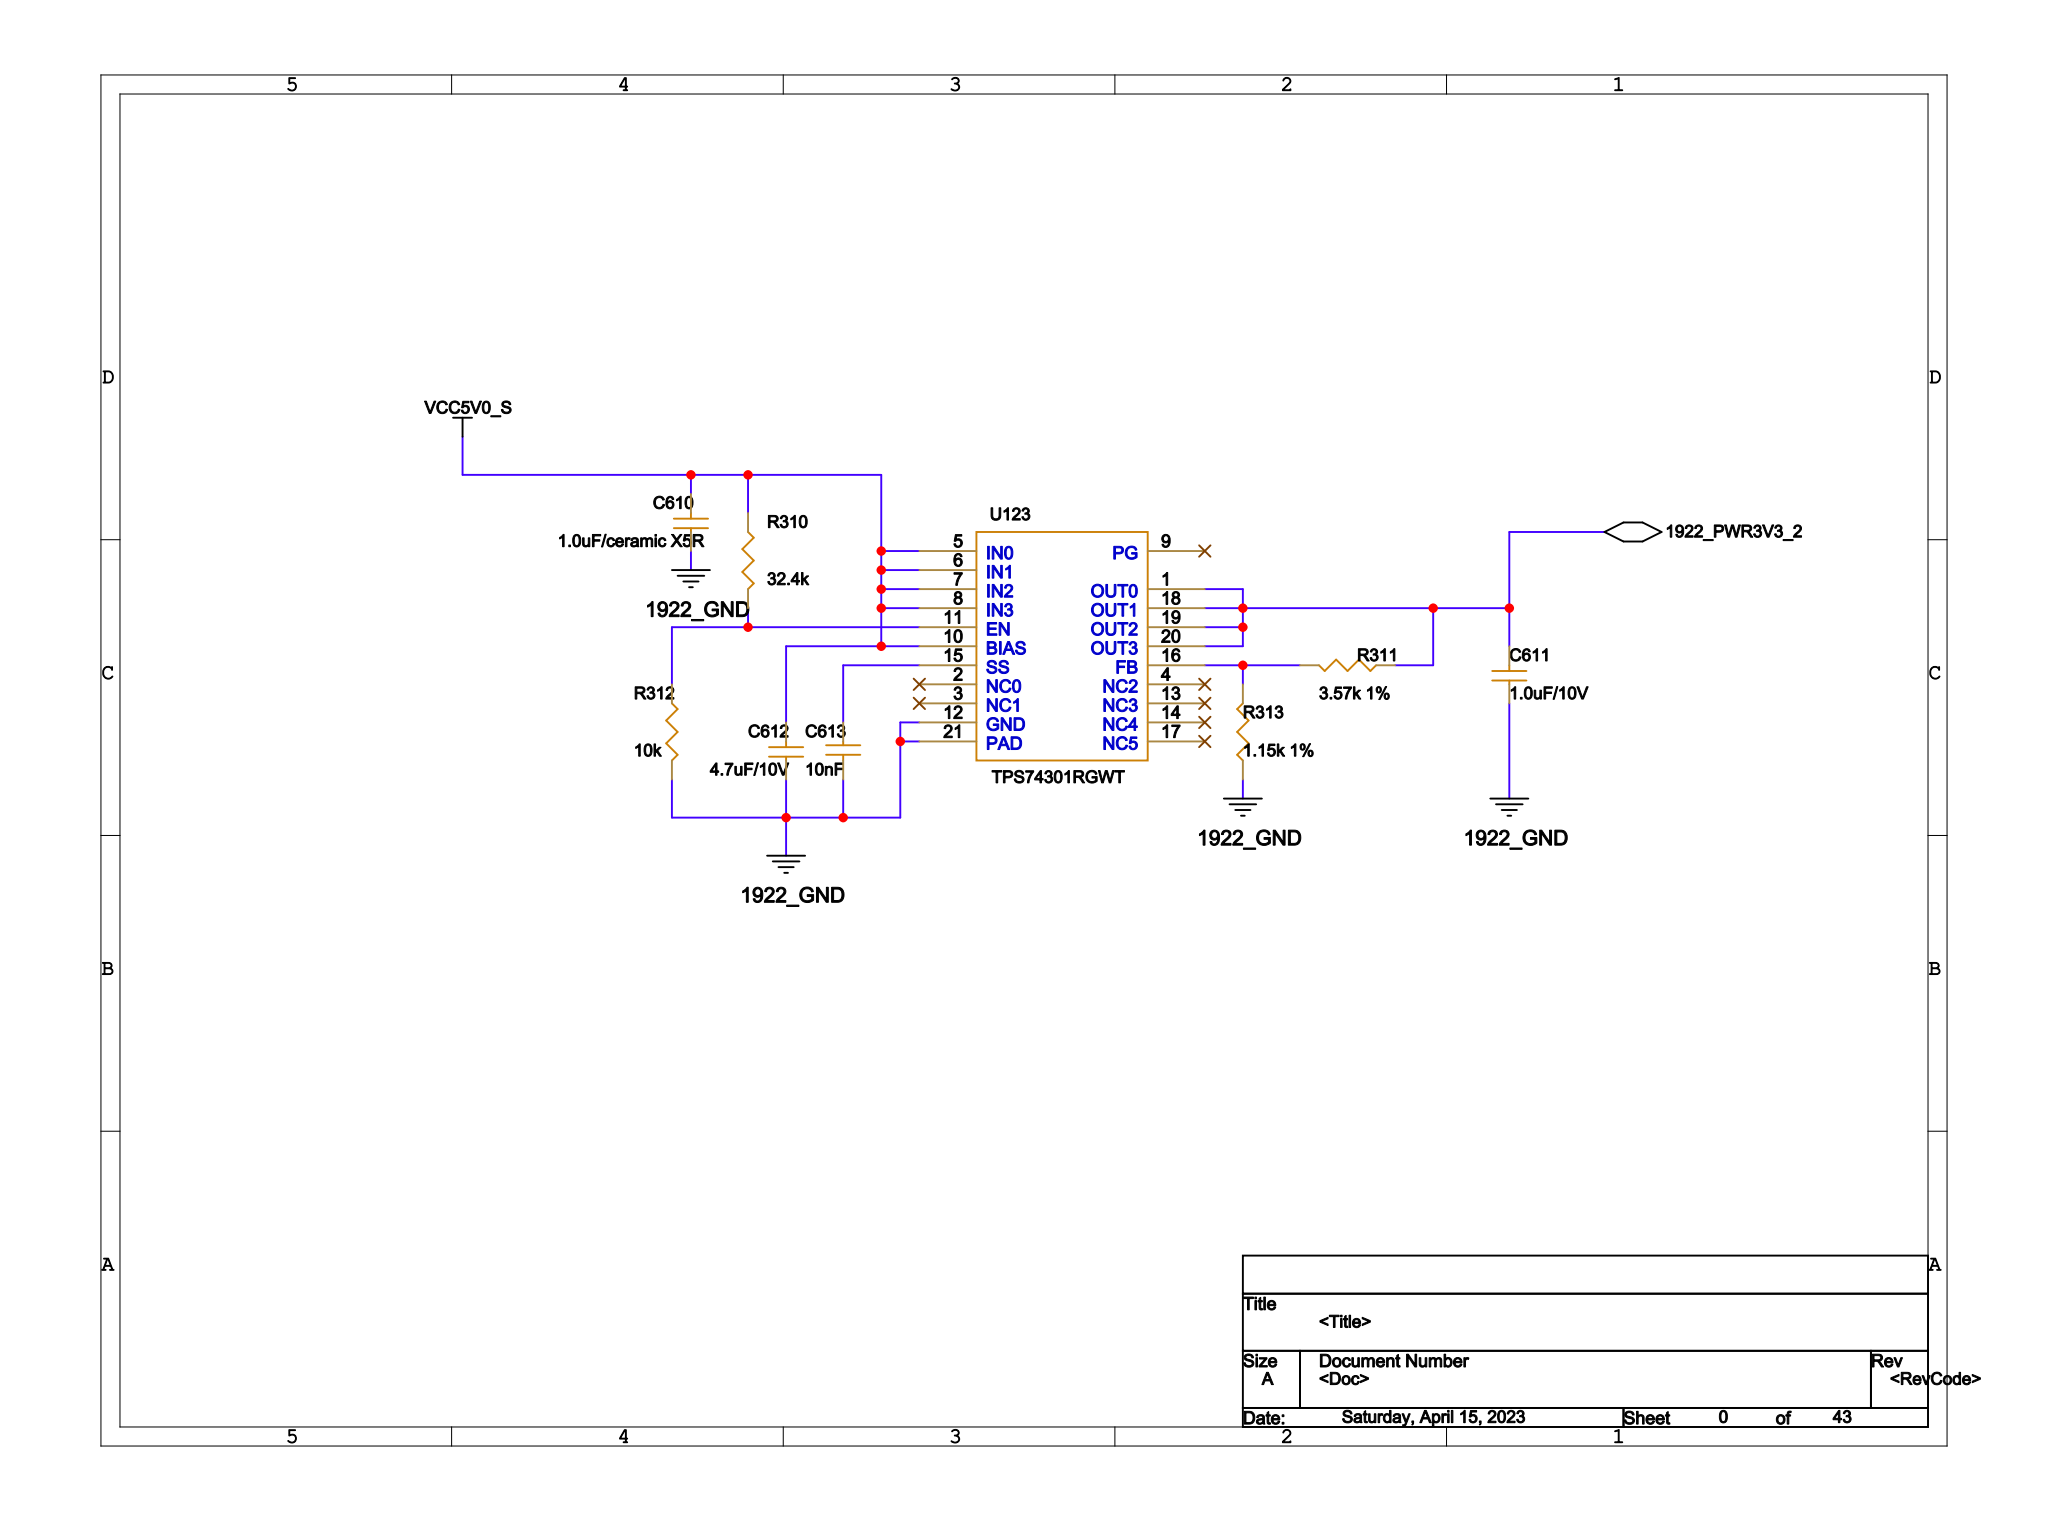Circuit board | Cadence Allegro | 1034 parts | 912 nets | one sheet of the schematic
Parts on this sheet (reference | value | footprint):
C610 | 1.0uF/ceramic X5R | C0402
C611 | 1.0uF/10V | C0402
C612 | 4.7uF/10V | C0402
C613 | 10nF | C0402
R310 | 32.4k | R0402
R311 | 3.57k 1% | R0402
R312 | 10k | R0402
R313 | 1.15k 1% | R0402
U123 | TPS74301RGWT | TPS74301_VQFN
Nets of these parts (net: part-pin ...):
VCC5V0_S: C610-2 C612-2 R310-1 U123-5 U123-6 U123-7 U123-8 U123-10
1922_GND: C610-1 C611-1 C612-1 C613-2 R312-2 R313-1 U123-12 U123-21
PWR1922_3V3_2: C611-2 R311-1 U123-1 U123-18 U123-19 U123-20
N14252006: C613-1 U123-15
N14251918: R310-2 R312-1 U123-11
N14252014: R311-2 R313-2 U123-16